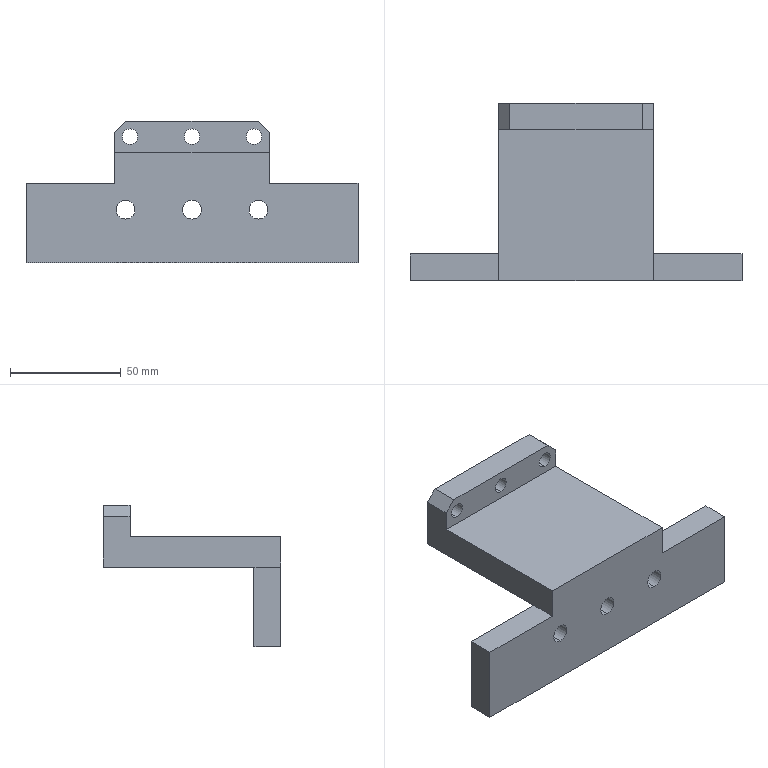NC program | NX | posted with a generic post | part box 150 x 80 x 64 mm
Lines 9556 to 10576 of 10576:
(FLOOR_WALL_1 , TOOL : D10)
N19104 T10 M6
N19106 G54
N19108 G17 G0 G90 X80.975 Y-21.86 B0. C0. S9500 M3
N19110 G43 Z30. H10
N19112 Z-26.5
N19114 G94 G1 Z-28. F1250.
N19116 X80.5 Y-22.134
N19118 G3 X80. Y-23. R1.
N19120 G1 Y-45.
N19122 X75.062
N19124 Y-23.
N19126 X70.125
N19128 Y-45.
N19130 X65.187
N19132 Y-23.
N19134 X60.25
N19136 Y-45.
N19138 X55.313
N19140 Y-23.
N19142 X50.375
N19144 Y-45.
N19146 X45.438
N19148 Y-23.
N19150 X40.5
N19152 Y-45.
N19154 G3 X41. Y-45.866 R1.
N19156 G1 X42.098 Y-46.5
N19158 Z-26.5
N19160 G0 Z30.
N19162 X41.598 Y-21.5
N19164 Z-26.5
N19166 G1 Z-28.
N19168 X40.5 Y-22.134
N19170 G3 X40. Y-23. R1.
N19172 G1 Y-45.
N19174 G3 X40.5 Y-45.866 R1.
N19176 G1 X41.598 Y-46.5
N19178 Z-26.5
N19180 G0 Z30.
N19182 X41.14 Y-45.975
N19184 Z-12.5
N19186 G1 Z-14.
N19188 X40.866 Y-45.5
N19190 G3 X40. Y-45. R1.
N19192 G1 X-40.
N19194 Y-40.179
N19196 X40.
N19198 Y-35.357
N19200 X-40.
N19202 Y-30.536
N19204 X40.
N19206 Y-25.714
N19208 X-40.
N19210 Y-20.893
N19212 X40.
N19214 Y-16.071
N19216 X-40.
N19218 Y-11.25
N19220 X40.
N19222 Y-6.429
N19224 X-40.
N19226 Y-1.607
N19228 X40.
N19230 Y3.214
N19232 X-40.
N19234 Y8.036
N19236 X40.
N19238 Y12.857
N19240 X-40.
N19242 Y17.679
N19244 X40.
N19246 Y22.5
N19248 X-40.
N19250 G3 X-40.866 Y22. R1.
N19252 G1 X-41.5 Y20.902
N19254 Z-12.5
N19256 G0 Z30.
N19258 X41.5 Y21.402
N19260 Z-12.5
N19262 G1 Z-14.
N19264 X40.866 Y22.5
N19266 G3 X40. Y23. R1.
N19268 G1 X-40.
N19270 G3 X-40.866 Y22.5 R1.
N19272 G1 X-41.5 Y21.402
N19274 Z-12.5
N19276 G0 Z30.
N19278 X-80.975 Y-46.14
N19280 Z-26.5
N19282 G1 Z-28.
N19284 X-80.5 Y-45.866
N19286 G3 X-80. Y-45. R1.
N19288 G1 Y-23.
N19290 X-75.062
N19292 Y-45.
N19294 X-70.125
N19296 Y-23.
N19298 X-65.188
N19300 Y-45.
N19302 X-60.25
N19304 Y-23.
N19306 X-55.313
N19308 Y-45.
N19310 X-50.375
N19312 Y-23.
N19314 X-45.438
N19316 Y-45.
N19318 X-40.5
N19320 Y-23.
N19322 G3 X-41. Y-22.134 R1.
N19324 G1 X-42.098 Y-21.5
N19326 Z-26.5
N19328 G0 Z30.
N19330 X-41.598 Y-46.5
N19332 Z-26.5
N19334 G1 Z-28.
N19336 X-40.5 Y-45.866
N19338 G3 X-40. Y-45. R1.
N19340 G1 Y-23.
N19342 G3 X-40.5 Y-22.134 R1.
N19344 G1 X-41.598 Y-21.5
N19346 Z-26.5
N19348 G0 Z30.
(ZLEVEL_PROFILE_COPY , TOOL : D10)
N19350 X76.622 Y-46.809
N19352 Z-14.475
N19354 G1 Z-15.975
N19356 X75.866 Y-45.5
N19358 G3 X75. Y-45. R1.
N19360 G1 X-75.
N19362 G2 X-80. Y-40. R5.
N19364 G1 Y-28.
N19366 G2 X-75. Y-23. R5.
N19368 G1 X-40.
N19370 Y40.
N19372 G2 X-35. Y45. R5.
N19374 G1 X35.
N19376 G2 X40. Y40. R5.
N19378 G1 Y-23.
N19380 X75.
N19382 G2 X80. Y-28. R5.
N19384 G1 Y-40.
N19386 G2 X75. Y-45. R5.
N19388 G3 X74.134 Y-45.5 R1.
N19390 G1 X73.268 Y-47.
N19392 Z-14.475
N19394 G0 Z30.
N19396 X76.622 Y-46.809
N19398 Z-30.45
N19400 G1 Z-31.95
N19402 X75.866 Y-45.5
N19404 G3 X75. Y-45. R1.
N19406 G1 X-75.
N19408 G2 X-80. Y-40. R5.
N19410 G1 Y-28.
N19412 G2 X-75. Y-23. R5.
N19414 G1 X-40.
N19416 Y40.
N19418 G2 X-35. Y45. R5.
N19420 G1 X35.
N19422 G2 X40. Y40. R5.
N19424 G1 Y-23.
N19426 X75.
N19428 G2 X80. Y-28. R5.
N19430 G1 Y-40.
N19432 G2 X75. Y-45. R5.
N19434 G3 X74.134 Y-45.5 R1.
N19436 G1 X73.268 Y-47.
N19438 Z-30.45
N19440 G0 Z30.
N19442 X76.622 Y-46.809
N19444 Z-46.425
N19446 G1 Z-47.925
N19448 X75.866 Y-45.5
N19450 G3 X75. Y-45. R1.
N19452 G1 X-75.
N19454 G2 X-80. Y-40. R5.
N19456 G1 Y-28.
N19458 G2 X-75. Y-23. R5.
N19460 G1 X-40.
N19462 Y40.
N19464 G2 X-35. Y45. R5.
N19466 G1 X35.
N19468 G2 X40. Y40. R5.
N19470 G1 Y-23.
N19472 X75.
N19474 G2 X80. Y-28. R5.
N19476 G1 Y-40.
N19478 G2 X75. Y-45. R5.
N19480 G3 X74.134 Y-45.5 R1.
N19482 G1 X73.268 Y-47.
N19484 Z-46.425
N19486 G0 Z30.
N19488 X76.622 Y-46.809
N19490 Z-62.4
N19492 G1 Z-63.9
N19494 X75.866 Y-45.5
N19496 G3 X75. Y-45. R1.
N19498 G1 X-75.
N19500 G2 X-80. Y-40. R5.
N19502 G1 Y-28.
N19504 G2 X-75. Y-23. R5.
N19506 G1 X-40.
N19508 Y40.
N19510 G2 X-35. Y45. R5.
N19512 G1 X35.
N19514 G2 X40. Y40. R5.
N19516 G1 Y-23.
N19518 X75.
N19520 G2 X80. Y-28. R5.
N19522 G1 Y-40.
N19524 G2 X75. Y-45. R5.
N19526 G3 X74.134 Y-45.5 R1.
N19528 G1 X73.268 Y-47.
N19530 Z-62.4
N19532 G0 Z30.
N19534 M5
(ZLEVEL_PROFILE_1 , TOOL : D4R0.5)
N19536 T05 M6
N19538 G54
N19540 G17 G0 G90 X32.492 Y41.116 B0. C0. S9500 M3
N19542 G43 Z30. H5
N19544 Z1.429
N19546 G94 G1 Z-0.071 F1000.
N19548 X31.977 Y40.819
N19550 G3 X31.777 Y40.473 R0.4
N19552 G1 X31.778 Y27.527 F2500.
N19554 X31.813 Z-0.106
N19556 X31.848 Z-0.141
N19558 Y40.473
N19560 X31.884 Z-0.177
N19562 X31.919 Y40.474 Z-0.212
N19564 Y40.
N19566 Y28.
N19568 Y27.526
N19570 X31.955 Z-0.247
N19572 X31.99 Z-0.283
N19574 Y28.
N19576 Y40.
N19578 X31.989 Y40.474
N19580 X32.025 Z-0.318
N19582 X32.06 Y40.475 Z-0.354
N19584 X32.061 Y40.
N19586 Y28.
N19588 Y27.525
N19590 X32.096 Z-0.389
N19592 X32.131 Z-0.424
N19594 Y28.
N19596 Y40.
N19598 Y40.475
N19600 X32.167 Z-0.46
N19602 X32.202 Y40.476 Z-0.495
N19604 Y40.
N19606 Y28.
N19608 Y27.524
N19610 X32.237 Z-0.53
N19612 X32.273 Z-0.566
N19614 Y28.
N19616 Y40.
N19618 X32.272 Y40.476
N19620 X32.308 Z-0.601
N19622 X32.343 Y40.477 Z-0.636
N19624 X32.344 Y40.
N19626 Y28.
N19628 X32.343 Y27.523
N19630 X32.379 Z-0.672
N19632 X32.414 Z-0.707
N19634 Y28.
N19636 Y40.
N19638 Y40.477
N19640 X32.45 Z-0.742
N19642 X32.484 Y40.478 Z-0.778
N19644 X32.485 Y40.
N19646 Y28.
N19648 Y27.522
N19650 X32.52 Z-0.813
N19652 X32.556 Z-0.849
N19654 Y28.
N19656 Y40.
N19658 X32.555 Y40.478
N19660 X32.591 Z-0.884
N19662 X32.626 Y40.479 Z-0.919
N19664 Y40.
N19666 Y28.
N19668 Y27.521
N19670 X32.662 Z-0.955
N19672 X32.697 Z-0.99
N19674 Y28.
N19676 Y40.
N19678 X32.696 Y40.479
N19680 X32.732 Z-1.025
N19682 X32.767 Y40.48 Z-1.061
N19684 X32.768 Y40.
N19686 Y28.
N19688 Y27.52
N19690 X32.803 Z-1.096
N19692 X32.838 Z-1.131
N19694 Y28.
N19696 Y40.
N19698 Y40.48
N19700 X32.874 Z-1.167
N19702 X32.908 Y40.481 Z-1.202
N19704 X32.909 Y40.
N19706 Y28.
N19708 Y27.519
N19710 X32.945 Z-1.237
N19712 X32.98 Z-1.273
N19714 Y28.
N19716 Y40.
N19718 X32.979 Y40.481
N19720 X33.015 Z-1.308
N19722 X33.05 Y40.482 Z-1.344
N19724 X33.051 Y40.
N19726 Y28.
N19728 Y27.518
N19730 X33.086 Z-1.379
N19732 X33.121 Z-1.414
N19734 Y28.
N19736 Y40.
N19738 X33.12 Y40.482
N19740 X33.157 Z-1.45
N19742 X33.191 Z-1.485
N19744 X33.192 Y40.
N19746 Y28.
N19748 Y27.518
N19750 X33.227 Z-1.52
N19752 X33.263 Z-1.556
N19754 Y28.
N19756 Y40.
N19758 X33.262 Y40.482
N19760 X33.298 Y40.483 Z-1.591
N19762 X33.333 Z-1.626
N19764 Y40.
N19766 Y28.
N19768 Y27.517
N19770 X33.369 Z-1.662
N19772 X33.404 Z-1.697
N19774 Y28.
N19776 Y40.
N19778 X33.403 Y40.483
N19780 X33.44 Z-1.732
N19782 X33.474 Z-1.768
N19784 X33.475 Y40.
N19786 Y28.
N19788 Y27.517
N19790 X33.51 Z-1.803
N19792 X33.546 Z-1.838
N19794 Y28.
N19796 Y40.
N19798 X33.545 Y40.483
N19800 X33.581 Z-1.874
N19802 X33.615 Y40.484 Z-1.909
N19804 X33.616 Y40.
N19806 Y28.
N19808 Y27.516
N19810 X33.652 Z-1.945
N19812 X33.687 Z-1.98
N19814 Y28.
N19816 Y40.
N19818 X33.686 Y40.484
N19820 X33.722 Z-2.015
N19822 X33.757 Z-2.051
N19824 X33.758 Y40.
N19826 Y28.
N19828 Y27.516
N19830 X33.793 Z-2.086
N19832 X33.828 Z-2.121
N19834 Y28.
N19836 Y40.
N19838 X33.827 Y40.484
N19840 X33.864 Z-2.157
N19842 X33.898 Y40.485 Z-2.192
N19844 X33.899 Y40.
N19846 Y28.
N19848 Y27.516
N19850 X33.934 Y27.515 Z-2.227
N19852 X33.97 Z-2.263
N19854 Y28.
N19856 Y40.
N19858 X33.969 Y40.485
N19860 X34.005 Z-2.298
N19862 X34.039 Z-2.333
N19864 X34.041 Y40.
N19866 Y28.
N19868 Y27.515
N19870 X34.076 Z-2.369
N19872 X34.111 Z-2.404
N19874 Y28.
N19876 Y40.
N19878 X34.11 Y40.485
N19880 X34.147 Z-2.44
N19882 X34.181 Z-2.475
N19884 X34.182 Y40.
N19886 Y28.
N19888 Y27.515
N19890 X34.217 Z-2.51
N19892 X34.253 Z-2.546
N19894 Y28.
N19896 Y40.
N19898 X34.252 Y40.485
N19900 X34.288 Z-2.581
N19902 X34.322 Y40.486 Z-2.616
N19904 X34.323 Y40.
N19906 Y28.
N19908 Y27.514
N19910 X34.359 Z-2.652
N19912 X34.394 Z-2.687
N19914 Y28.
N19916 Y40.
N19918 X34.393 Y40.486
N19920 X34.429 Z-2.722
N19922 X34.464 Z-2.758
N19924 X34.465 Y40.
N19926 Y28.
N19928 Y27.514
N19930 X34.5 Z-2.793
N19932 X34.536 Y27.515 Z-2.828
N19934 Y28.
N19936 Y40.
N19938 X34.534 Y40.485
N19940 X34.571 Z-2.864
N19942 X34.605 Z-2.899
N19944 X34.606 Y40.
N19946 Y28.
N19948 Y27.515
N19950 X34.642 Z-2.934
N19952 X34.677 Z-2.97
N19954 Y28.
N19956 Y40.
N19958 X34.676 Y40.485
N19960 X34.712 Z-3.005
N19962 X34.747 Z-3.041
N19964 X34.748 Y40.
N19966 Y28.
N19968 Y27.515
N19970 X34.783 Z-3.076
N19972 X34.818 Z-3.111
N19974 Y28.
N19976 Y40.
N19978 X34.817 Y40.484
N19980 X34.854 Z-3.147
N19982 X34.888 Z-3.182
N19984 X34.889 Y40.
N19986 Y28.
N19988 Y27.516
N19990 X34.924 Z-3.217
N19992 X34.96 Z-3.253
N19994 Y28.
N19996 Y40.
N19998 X34.959 Y40.484
N20000 X34.995 Z-3.288
N20002 X35.029 Z-3.323
N20004 X35.031 Y40.
N20006 Y28.
N20008 Y27.516
N20010 X35.066 Z-3.359
N20012 X35.101 Z-3.394
N20014 Y28.
N20016 Y40.
N20018 X35.1 Y40.484
N20020 X35.137 Z-3.429
N20022 X35.171 Y40.483 Z-3.465
N20024 X35.172 Y40.
N20026 Y28.
N20028 Y27.517
N20030 X35.207 Z-3.5
N20032 X35.243 Z-3.536
N20034 Y28.
N20036 Y40.
N20038 X35.242 Y40.483
N20040 X35.278 Z-3.571
N20042 X35.312 Z-3.606
N20044 X35.313 Y40.
N20046 Y28.
N20048 Y27.517
N20050 X35.349 Z-3.642
N20052 X35.384 Z-3.677
N20054 Y28.
N20056 Y40.
N20058 X35.383 Y40.483
N20060 X35.419 Z-3.712
N20062 X35.454 Y40.482 Z-3.748
N20064 X35.455 Y40.
N20066 Y28.
N20068 Y27.518
N20070 X35.49 Z-3.783
N20072 X35.525 Z-3.818
N20074 Y28.
N20076 Y40.
N20078 Y40.482
N20080 X35.561 Z-3.854
N20082 X35.595 Z-3.889
N20084 X35.596 Y40.
N20086 Y28.
N20088 Y27.518
N20090 X35.632 Z-3.924
N20092 X35.667 Y27.519 Z-3.96
N20094 Y28.
N20096 Y40.
N20098 X35.666 Y40.481
N20100 X35.702 Z-3.995
N20102 X35.737 Z-4.031
N20104 X35.738 Y40.
N20106 Y28.
N20108 Y27.519
N20110 X35.773 Z-4.066
N20112 X35.808 Z-4.101
N20114 Y28.
N20116 Y40.
N20118 X35.807 Y40.481
N20120 X35.844 Y40.48 Z-4.137
N20122 X35.878 Z-4.172
N20124 X35.879 Y40.
N20126 Y28.
N20128 Y27.52
N20130 X35.914 Z-4.207
N20132 X35.95 Z-4.243
N20134 Y28.
N20136 Y40.
N20138 X35.949 Y40.48
N20140 X35.985 Y40.479 Z-4.278
N20142 X36.02 Z-4.313
N20144 Y40.
N20146 Y28.
N20148 Y27.521
N20150 X36.056 Z-4.349
N20152 X36.091 Z-4.384
N20154 Y28.
N20156 Y40.
N20158 X36.09 Y40.479
N20160 X36.127 Y40.478 Z-4.419
N20162 X36.161 Z-4.455
N20164 X36.162 Y40.
N20166 Y28.
N20168 Y27.522
N20170 X36.197 Z-4.49
N20172 X36.233 Z-4.525
N20174 Y28.
N20176 Y40.
N20178 X36.232 Y40.478
N20180 X36.268 Y40.477 Z-4.561
N20182 X36.303 Z-4.596
N20184 Y40.
N20186 Y28.
N20188 Y27.523
N20190 X36.339 Z-4.632
N20192 X36.374 Z-4.667
N20194 Y28.
N20196 Y40.
N20198 X36.373 Y40.477
N20200 X36.409 Y40.476 Z-4.702
N20202 X36.444 Z-4.738
N20204 X36.445 Y40.
N20206 Y28.
N20208 Y27.524
N20210 X36.48 Z-4.773
N20212 X36.515 Z-4.808
N20214 Y28.
N20216 Y40.
N20218 Y40.476
N20220 X36.551 Y40.475 Z-4.844
N20222 X36.586 Z-4.879
N20224 Y40.
N20226 Y28.
N20228 Y27.525
N20230 X36.622 Z-4.914
N20232 X36.657 Y27.526 Z-4.95
N20234 Y28.
N20236 Y40.
N20238 X36.656 Y40.475
N20240 X36.692 Y40.474 Z-4.985
N20242 X36.727 Z-5.02
N20244 X36.728 Y40.
N20246 Y28.
N20248 Y27.526
N20250 X36.763 Z-5.056
N20252 X36.798 Y27.527 Z-5.091
N20254 Y28.
N20256 Y40.
N20258 Y40.474
N20260 X36.834 Y40.473 Z-5.127
N20262 X36.869 Z-5.162
N20264 Y27.527
N20266 X36.904 Y27.533 Z-5.197
N20268 X36.94 Y27.539 Z-5.233
N20270 X36.939 Y40.472
N20272 X36.973 Z-5.266
N20274 X37.006 Y40.471 Z-5.299
N20276 Y27.608
N20278 X37.073 Y27.677 Z-5.366
N20280 Y40.47
N20282 X37.107 Y40.469 Z-5.4
N20284 X37.14 Z-5.433
N20286 Y27.747
N20288 G3 X37.34 Y27.4 R0.4
N20290 G1 X37.902 Y27.076
N20292 Z-3.933
N20294 G0 Z30.
N20296 X-32.498 Y26.881
N20298 Z1.429
N20300 G1 Z-0.071 F1000.
N20302 X-31.978 Y27.181
N20304 G3 X-31.778 Y27.527 R0.4
N20306 G1 X-31.777 Y40.473 F2500.
N20308 X-31.813 Z-0.106
N20310 X-31.848 Z-0.141
N20312 Y27.527
N20314 X-31.884 Z-0.177
N20316 X-31.919 Y27.526 Z-0.212
N20318 Y28.
N20320 Y40.
N20322 Y40.474
N20324 X-31.955 Z-0.247
N20326 X-31.989 Z-0.283
N20328 X-31.99 Y40.
N20330 Y28.
N20332 Y27.526
N20334 X-32.025 Z-0.318
N20336 X-32.061 Y27.525 Z-0.354
N20338 Y28.
N20340 Y40.
N20342 X-32.06 Y40.475
N20344 X-32.096 Z-0.389
N20346 X-32.131 Z-0.424
N20348 Y40.
N20350 Y28.
N20352 Y27.525
N20354 X-32.167 Z-0.46
N20356 X-32.202 Y27.524 Z-0.495
N20358 Y28.
N20360 Y40.
N20362 Y40.476
N20364 X-32.237 Z-0.53
N20366 X-32.272 Z-0.566
N20368 X-32.273 Y40.
N20370 Y28.
N20372 Y27.524
N20374 X-32.308 Z-0.601
N20376 X-32.343 Y27.523 Z-0.636
N20378 X-32.344 Y28.
N20380 Y40.
N20382 X-32.343 Y40.477
N20384 X-32.379 Z-0.672
N20386 X-32.414 Z-0.707
N20388 Y40.
N20390 Y28.
N20392 Y27.523
N20394 X-32.45 Z-0.742
N20396 X-32.485 Y27.522 Z-0.778
N20398 Y28.
N20400 Y40.
N20402 X-32.484 Y40.478
N20404 X-32.52 Z-0.813
N20406 X-32.555 Z-0.849
N20408 X-32.556 Y40.
N20410 Y28.
N20412 Y27.522
N20414 X-32.591 Z-0.884
N20416 X-32.626 Y27.521 Z-0.919
N20418 Y28.
N20420 Y40.
N20422 Y40.479
N20424 X-32.662 Z-0.955
N20426 X-32.696 Z-0.99
N20428 X-32.697 Y40.
N20430 Y28.
N20432 Y27.521
N20434 X-32.732 Z-1.025
N20436 X-32.768 Y27.52 Z-1.061
N20438 Y28.
N20440 Y40.
N20442 X-32.767 Y40.48
N20444 X-32.803 Z-1.096
N20446 X-32.838 Z-1.131
N20448 Y40.
N20450 Y28.
N20452 Y27.52
N20454 X-32.874 Z-1.167
N20456 X-32.909 Y27.519 Z-1.202
N20458 Y28.
N20460 Y40.
N20462 X-32.908 Y40.481
N20464 X-32.945 Z-1.237
N20466 X-32.979 Z-1.273
N20468 X-32.98 Y40.
N20470 Y28.
N20472 Y27.519
N20474 X-33.015 Z-1.308
N20476 X-33.051 Y27.518 Z-1.344
N20478 Y28.
N20480 Y40.
N20482 X-33.05 Y40.482
N20484 X-33.086 Z-1.379
N20486 X-33.12 Z-1.414
N20488 X-33.121 Y40.
N20490 Y28.
N20492 Y27.518
N20494 X-33.157 Z-1.45
N20496 X-33.192 Z-1.485
N20498 Y28.
N20500 Y40.
N20502 X-33.191 Y40.482
N20504 X-33.227 Z-1.52
N20506 X-33.262 Z-1.556
N20508 X-33.263 Y40.
N20510 Y28.
N20512 Y27.518
N20514 X-33.298 Y27.517 Z-1.591
N20516 X-33.333 Z-1.626
N20518 Y28.
N20520 Y40.
N20522 Y40.483
N20524 X-33.369 Z-1.662
N20526 X-33.403 Z-1.697
N20528 X-33.404 Y40.
N20530 Y28.
N20532 Y27.517
N20534 X-33.44 Z-1.732
N20536 X-33.475 Z-1.768
N20538 Y28.
N20540 Y40.
N20542 X-33.474 Y40.483
N20544 X-33.51 Z-1.803
N20546 X-33.545 Z-1.838
N20548 X-33.546 Y40.
N20550 Y28.
N20552 Y27.517
N20554 X-33.581 Y27.516 Z-1.874
N20556 X-33.616 Z-1.909
N20558 Y28.
N20560 Y40.
N20562 X-33.615 Y40.484
N20564 X-33.652 Z-1.945
N20566 X-33.686 Z-1.98
N20568 X-33.687 Y40.
N20570 Y28.
N20572 Y27.516
N20574 X-33.722 Z-2.015
N20576 X-33.758 Z-2.051
N20578 Y28.
N20580 Y40.
N20582 X-33.757 Y40.484
N20584 X-33.793 Z-2.086
N20586 X-33.827 Z-2.121
N20588 X-33.828 Y40.
N20590 Y28.
N20592 Y27.516
N20594 X-33.864 Z-2.157
N20596 X-33.899 Z-2.192
N20598 Y28.
N20600 Y40.
N20602 X-33.898 Y40.485
N20604 X-33.934 Z-2.227
N20606 X-33.969 Z-2.263
N20608 X-33.97 Y40.
N20610 Y28.
N20612 Y27.515
N20614 X-34.005 Z-2.298
N20616 X-34.041 Z-2.333
N20618 Y28.
N20620 Y40.
N20622 X-34.039 Y40.485
N20624 X-34.076 Z-2.369
N20626 X-34.11 Z-2.404
N20628 X-34.111 Y40.
N20630 Y28.
N20632 Y27.515
N20634 X-34.147 Y27.514 Z-2.44
N20636 X-34.182 Z-2.475
N20638 Y28.
N20640 Y40.
N20642 X-34.181 Y40.485
N20644 X-34.217 Z-2.51
N20646 X-34.252 Z-2.546
N20648 X-34.253 Y40.
N20650 Y28.
N20652 Y27.514
N20654 X-34.288 Z-2.581
N20656 X-34.323 Z-2.616
N20658 Y28.
N20660 Y40.
N20662 X-34.322 Y40.486
N20664 X-34.359 Z-2.652
N20666 X-34.393 Z-2.687
N20668 X-34.394 Y40.
N20670 Y28.
N20672 Y27.514
N20674 X-34.429 Z-2.722
N20676 X-34.465 Z-2.758
N20678 Y28.
N20680 Y40.
N20682 X-34.464 Y40.486
N20684 X-34.5 Y40.485 Z-2.793
N20686 X-34.534 Z-2.828
N20688 X-34.536 Y40.
N20690 Y28.
N20692 Y27.514
N20694 X-34.571 Z-2.864
N20696 X-34.606 Y27.515 Z-2.899
N20698 Y28.
N20700 Y40.
N20702 X-34.605 Y40.485
N20704 X-34.642 Z-2.934
N20706 X-34.676 Z-2.97
N20708 X-34.677 Y40.
N20710 Y28.
N20712 Y27.515
N20714 X-34.712 Z-3.005
N20716 X-34.748 Z-3.041
N20718 Y28.
N20720 Y40.
N20722 X-34.747 Y40.485
N20724 X-34.783 Z-3.076
N20726 X-34.817 Y40.484 Z-3.111
N20728 X-34.818 Y40.
N20730 Y28.
N20732 Y27.515
N20734 X-34.854 Y27.516 Z-3.147
N20736 X-34.889 Z-3.182
N20738 Y28.
N20740 Y40.
N20742 X-34.888 Y40.484
N20744 X-34.924 Z-3.217
N20746 X-34.959 Z-3.253
N20748 X-34.96 Y40.
N20750 Y28.
N20752 Y27.516
N20754 X-34.995 Z-3.288
N20756 X-35.031 Z-3.323
N20758 Y28.
N20760 Y40.
N20762 X-35.029 Y40.484
N20764 X-35.066 Z-3.359
N20766 X-35.1 Z-3.394
N20768 X-35.101 Y40.
N20770 Y28.
N20772 Y27.516
N20774 X-35.137 Z-3.429
N20776 X-35.172 Y27.517 Z-3.465
N20778 Y28.
N20780 Y40.
N20782 X-35.171 Y40.483
N20784 X-35.207 Z-3.5
N20786 X-35.242 Z-3.536
N20788 X-35.243 Y40.
N20790 Y28.
N20792 Y27.517
N20794 X-35.278 Z-3.571
N20796 X-35.313 Z-3.606
N20798 Y28.
N20800 Y40.
N20802 X-35.312 Y40.483
N20804 X-35.349 Z-3.642
N20806 X-35.383 Z-3.677
N20808 X-35.384 Y40.
N20810 Y28.
N20812 Y27.517
N20814 X-35.419 Z-3.712
N20816 X-35.455 Y27.518 Z-3.748
N20818 Y28.
N20820 Y40.
N20822 X-35.454 Y40.482
N20824 X-35.49 Z-3.783
N20826 X-35.525 Z-3.818
N20828 Y40.
N20830 Y28.
N20832 Y27.518
N20834 X-35.561 Z-3.854
N20836 X-35.596 Z-3.889
N20838 Y28.
N20840 Y40.
N20842 X-35.595 Y40.482
N20844 X-35.632 Z-3.924
N20846 X-35.666 Y40.481 Z-3.96
N20848 X-35.667 Y40.
N20850 Y28.
N20852 Y27.519
N20854 X-35.702 Z-3.995
N20856 X-35.738 Z-4.031
N20858 Y28.
N20860 Y40.
N20862 X-35.737 Y40.481
N20864 X-35.773 Z-4.066
N20866 X-35.807 Z-4.101
N20868 X-35.808 Y40.
N20870 Y28.
N20872 Y27.519
N20874 X-35.844 Y27.52 Z-4.137
N20876 X-35.879 Z-4.172
N20878 Y28.
N20880 Y40.
N20882 X-35.878 Y40.48
N20884 X-35.914 Z-4.207
N20886 X-35.949 Z-4.243
N20888 X-35.95 Y40.
N20890 Y28.
N20892 Y27.52
N20894 X-35.985 Y27.521 Z-4.278
N20896 X-36.02 Z-4.313
N20898 Y28.
N20900 Y40.
N20902 Y40.479
N20904 X-36.056 Z-4.349
N20906 X-36.09 Z-4.384
N20908 X-36.091 Y40.
N20910 Y28.
N20912 Y27.521
N20914 X-36.127 Y27.522 Z-4.419
N20916 X-36.162 Z-4.455
N20918 Y28.
N20920 Y40.
N20922 X-36.161 Y40.478
N20924 X-36.197 Z-4.49
N20926 X-36.232 Z-4.525
N20928 X-36.233 Y40.
N20930 Y28.
N20932 Y27.522
N20934 X-36.268 Y27.523 Z-4.561
N20936 X-36.303 Z-4.596
N20938 Y28.
N20940 Y40.
N20942 Y40.477
N20944 X-36.339 Z-4.632
N20946 X-36.373 Z-4.667
N20948 X-36.374 Y40.
N20950 Y28.
N20952 Y27.523
N20954 X-36.409 Y27.524 Z-4.702
N20956 X-36.445 Z-4.738
N20958 Y28.
N20960 Y40.
N20962 X-36.444 Y40.476
N20964 X-36.48 Z-4.773
N20966 X-36.515 Z-4.808
N20968 Y40.
N20970 Y28.
N20972 Y27.524
N20974 X-36.551 Y27.525 Z-4.844
N20976 X-36.586 Z-4.879
N20978 Y28.
N20980 Y40.
N20982 Y40.475
N20984 X-36.622 Z-4.914
N20986 X-36.656 Z-4.95
N20988 X-36.657 Y40.
N20990 Y28.
N20992 Y27.526
N20994 X-36.692 Z-4.985
N20996 X-36.728 Z-5.02
N20998 Y28.
N21000 Y40.
N21002 X-36.727 Y40.474
N21004 X-36.763 Z-5.056
N21006 X-36.798 Z-5.091
N21008 Y40.
N21010 Y28.
N21012 Y27.527
N21014 X-36.834 Z-5.127
N21016 X-36.869 Z-5.162
N21018 Y40.473
N21020 X-36.904 Z-5.197
N21022 X-36.939 Y40.472 Z-5.233
N21024 X-36.94 Y27.539
N21026 X-37.006 Y27.608 Z-5.299
N21028 Y40.471
N21030 X-37.04 Z-5.333
N21032 X-37.073 Y40.47 Z-5.366
N21034 Y27.677
N21036 X-37.14 Y27.747 Z-5.433
N21038 Y40.469
N21040 G3 X-37.34 Y40.815 R0.4
N21042 G1 X-37.859 Y41.115
N21044 Z-3.933
N21046 G0 Z30.
N21048 M5
(PLANAR_MILL , TOOL : D6A45)
N21050 T07 M6
N21052 G54
N21054 G17 G0 G90 X0. Y24.1 B0. C0. S9500 M3
N21056 G43 Z30. H7
N21058 Z2.
N21060 G94 G1 Z-1. F1250.
N21062 Y27.1
N21064 X-34.9
N21066 G2 X-35.9 Y28.1 R1.
N21068 G1 Y39.9
N21070 G2 X-34.9 Y40.9 R1.
N21072 G1 X34.9
N21074 G2 X35.9 Y39.9 R1.
N21076 G1 Y28.1
N21078 G2 X34.9 Y27.1 R1.
N21080 G1 X0.
N21082 Y24.1
N21084 Z2.
N21086 G0 Z30.
(PLANAR_MILL_COPY , TOOL : D6A45)
N21088 X38.9 Y22.8
N21090 Z-12.
N21092 G1 Z-15.
N21094 X35.9 Y24.618
N21096 Y-39.9
N21098 G2 X34.9 Y-40.9 R1.
N21100 G1 X-34.9
N21102 G2 X-35.9 Y-39.9 R1.
N21104 G1 Y24.618
N21106 X-38.9 Y22.8
N21108 Z-12.
N21110 G0 Z30.
N21112 M5
N21114 M2